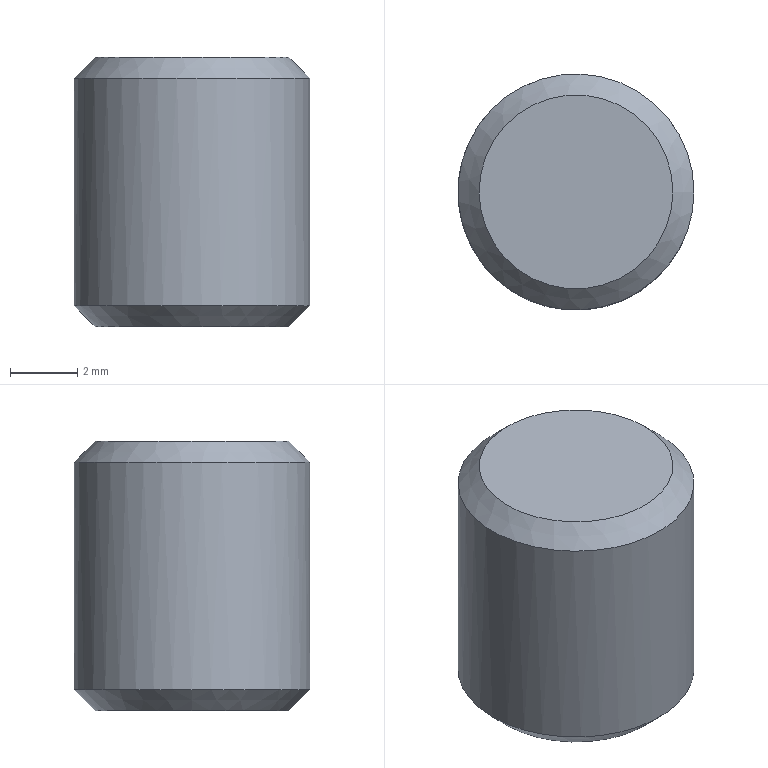Part | NX | features PG_666 2 | 1 solid | 5 faces | box 7 x 7 x 8 mm | volume 299.797 mm3 | plane 2 | cone 2 | cylinder 1 | commonest cylinder face diameters 7 x1
STEP:
#1=CARTESIAN_POINT('',(4300.21,-847.611,943.716));
#2=VERTEX_POINT('',#1);
#3=CARTESIAN_POINT('',(4297.335,-847.611,943.716));
#4=DIRECTION('',(0.,0.,1.));
#5=DIRECTION('',(1.,0.,0.));
#6=AXIS2_PLACEMENT_3D('',#3,#4,#5);
#7=CIRCLE('',#6,2.875);
#8=EDGE_CURVE('',#2,#2,#7,.T.);
#9=ORIENTED_EDGE('',*,*,#8,.T.);
#10=EDGE_LOOP('',(#9));
#11=FACE_BOUND('',#10,.T.);
#12=CARTESIAN_POINT('',(4297.335,-847.611,943.716));
#13=DIRECTION('',(0.,0.,1.));
#14=DIRECTION('',(1.,0.,0.));
#15=AXIS2_PLACEMENT_3D('',#12,#13,#14);
#16=PLANE('',#15);
#17=ADVANCED_FACE('',(#11),#16,.T.);
#18=CARTESIAN_POINT('',(4294.46,-847.611,935.716));
#19=VERTEX_POINT('',#18);
#20=CARTESIAN_POINT('',(4297.335,-847.611,935.716));
#21=DIRECTION('',(0.,0.,-1.));
#22=DIRECTION('',(-1.,0.,0.));
#23=AXIS2_PLACEMENT_3D('',#20,#21,#22);
#24=CIRCLE('',#23,2.875);
#25=EDGE_CURVE('',#19,#19,#24,.T.);
#26=ORIENTED_EDGE('',*,*,#25,.T.);
#27=EDGE_LOOP('',(#26));
#28=FACE_BOUND('',#27,.T.);
#29=CARTESIAN_POINT('',(4297.335,-847.611,935.716));
#30=DIRECTION('',(0.,0.,-1.));
#31=DIRECTION('',(-1.,0.,0.));
#32=AXIS2_PLACEMENT_3D('',#29,#30,#31);
#33=PLANE('',#32);
#34=ADVANCED_FACE('',(#28),#33,.T.);
#35=CARTESIAN_POINT('',(4293.835,-847.611,936.341));
#36=VERTEX_POINT('',#35);
#37=CARTESIAN_POINT('',(4297.335,-847.611,936.341));
#38=DIRECTION('',(0.,0.,-1.));
#39=DIRECTION('',(-1.,0.,0.));
#40=AXIS2_PLACEMENT_3D('',#37,#38,#39);
#41=CIRCLE('',#40,3.5);
#42=EDGE_CURVE('',#36,#36,#41,.F.);
#43=ORIENTED_EDGE('',*,*,#42,.T.);
#44=EDGE_LOOP('',(#43));
#45=FACE_BOUND('',#44,.T.);
#46=CARTESIAN_POINT('',(4300.835,-847.611,943.091));
#47=VERTEX_POINT('',#46);
#48=CARTESIAN_POINT('',(4297.335,-847.611,943.091));
#49=DIRECTION('',(0.,0.,1.));
#50=DIRECTION('',(1.,0.,0.));
#51=AXIS2_PLACEMENT_3D('',#48,#49,#50);
#52=CIRCLE('',#51,3.5);
#53=EDGE_CURVE('',#47,#47,#52,.F.);
#54=ORIENTED_EDGE('',*,*,#53,.T.);
#55=EDGE_LOOP('',(#54));
#56=FACE_BOUND('',#55,.T.);
#57=CARTESIAN_POINT('',(4297.335,-847.611,874.716));
#58=DIRECTION('',(0.,0.,1.));
#59=DIRECTION('',(1.,0.,0.));
#60=AXIS2_PLACEMENT_3D('',#57,#58,#59);
#61=CYLINDRICAL_SURFACE('',#60,3.5);
#62=ADVANCED_FACE('',(#45,#56),#61,.T.);
#63=ORIENTED_EDGE('',*,*,#25,.F.);
#64=EDGE_LOOP('',(#63));
#65=FACE_BOUND('',#64,.T.);
#66=ORIENTED_EDGE('',*,*,#42,.F.);
#67=EDGE_LOOP('',(#66));
#68=FACE_BOUND('',#67,.T.);
#69=CARTESIAN_POINT('',(4297.335,-847.611,936.341));
#70=DIRECTION('',(0.,0.,1.));
#71=DIRECTION('',(1.,0.,0.));
#72=AXIS2_PLACEMENT_3D('',#69,#70,#71);
#73=CONICAL_SURFACE('',#72,3.5,0.7854);
#74=ADVANCED_FACE('',(#65,#68),#73,.T.);
#75=ORIENTED_EDGE('',*,*,#8,.F.);
#76=EDGE_LOOP('',(#75));
#77=FACE_BOUND('',#76,.T.);
#78=ORIENTED_EDGE('',*,*,#53,.F.);
#79=EDGE_LOOP('',(#78));
#80=FACE_BOUND('',#79,.T.);
#81=CARTESIAN_POINT('',(4297.335,-847.611,943.091));
#82=DIRECTION('',(0.,0.,-1.));
#83=DIRECTION('',(-1.,0.,0.));
#84=AXIS2_PLACEMENT_3D('',#81,#82,#83);
#85=CONICAL_SURFACE('',#84,3.5,0.7854);
#86=ADVANCED_FACE('',(#77,#80),#85,.T.);
#87=CLOSED_SHELL('',(#17,#34,#62,#74,#86));
#88=MANIFOLD_SOLID_BREP('',#87);
#89=(LENGTH_UNIT()NAMED_UNIT(*)SI_UNIT(.MILLI.,.METRE.));
#90=UNCERTAINTY_MEASURE_WITH_UNIT(LENGTH_MEASURE(0.00001),#89,'','');
#91=(NAMED_UNIT(*)PLANE_ANGLE_UNIT()SI_UNIT($,.RADIAN.));
#92=(NAMED_UNIT(*)SI_UNIT($,.STERADIAN.)SOLID_ANGLE_UNIT());
#93=(GEOMETRIC_REPRESENTATION_CONTEXT(3)GLOBAL_UNCERTAINTY_ASSIGNED_CONTEXT((#90))GLOBAL_UNIT_ASSIGNED_CONTEXT((#89,#91,#92))REPRESENTATION_CONTEXT('',''));
#94=ADVANCED_BREP_SHAPE_REPRESENTATION('',(#88),#93);